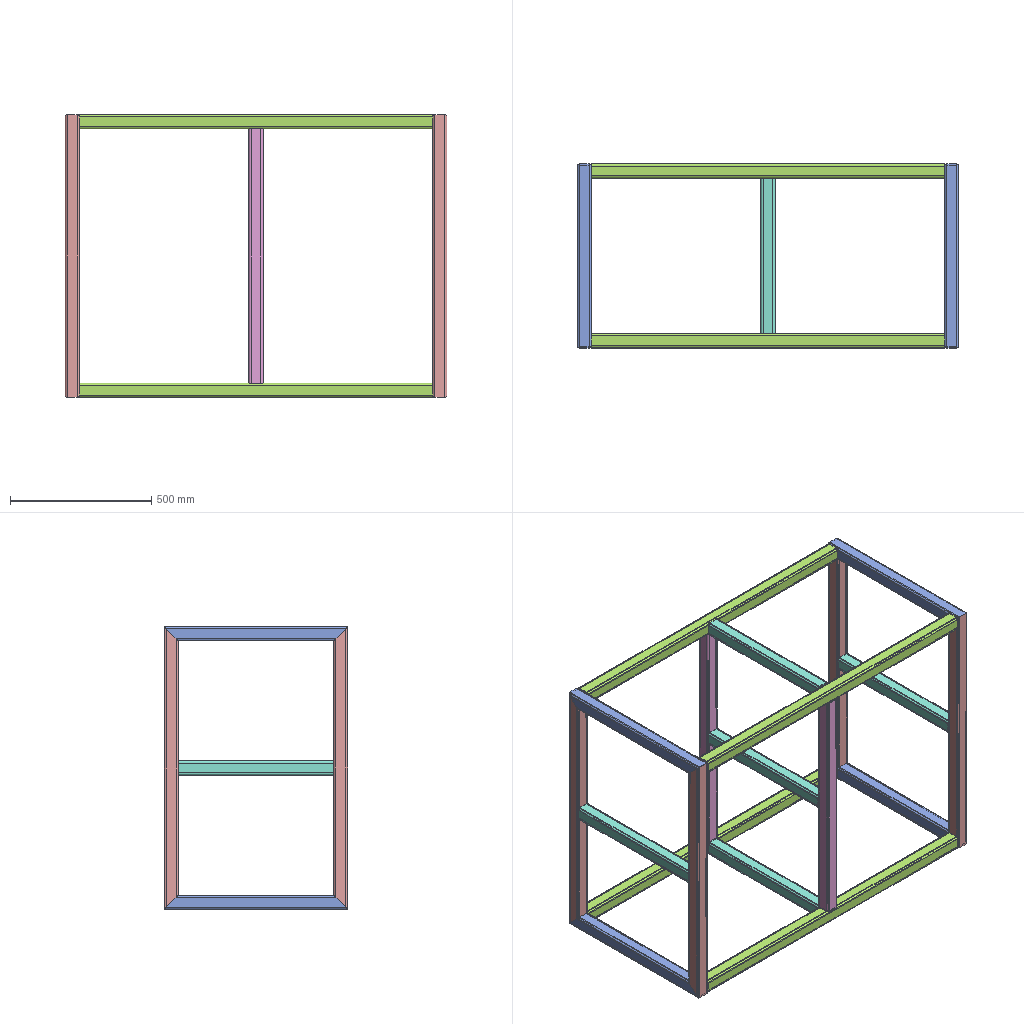Assembly | SolidWorks | 5 different items | 21 placed | box 1350 x 650 x 1000 mm
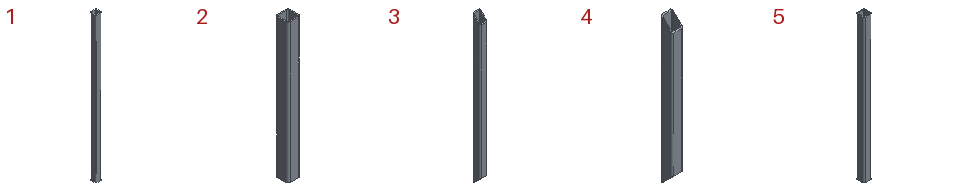Parts list (item | quantity | size | volume | features):
1 | x4 | 50 x 50 x 1250 mm | 868496 mm3 | features Extrusion 1
2 | x5 | 50 x 50 x 550 mm | 382138 mm3 | features Extrusion 1
3 | x6 | 50 x 50 x 1000 mm | 660057 mm3 | features Extrusion 1, ICE 1, MirrorPattern 1
4 | x4 | 50 x 50 x 650 mm | 416878 mm3 | features Extrusion 1, ICE 1, MirrorPattern 1
5 | x2 | 50 x 50 x 900 mm | 625317 mm3 | features Extrusion 1
Mates (type | each side: item.copy, entity, surface, feature):
Coincident | 3.1 face plane Boss-Extrude1 | 4.1 face plane Boss-Extrude1
Coincident | 3.1 face plane Mirror1 | 4.1 face plane Cut-Extrude1
Coincident | 3.1 edge | 4.1 edge
Coincident | 4.2 face plane Boss-Extrude1 | 1.1 face plane Boss-Extrude1 | 2 times
Coincident | 3.2 face plane Boss-Extrude1 | 1.1 face plane Boss-Extrude1
Coincident | 1.2 face plane Boss-Extrude1 | 5.1 face plane Boss-Extrude1 | 2 times
DistanceDim | 5.1 plane | 3.3 face plane Boss-Extrude1
Coincident | 3.4 face plane Boss-Extrude1 | 2.1 face plane Boss-Extrude1
Coincident | 3.2 face plane Boss-Extrude1 | 2.1 face plane Boss-Extrude1
DistanceDim | 2.1 plane | 4.2 face plane Boss-Extrude1
Coincident | 5.2 face plane Boss-Extrude1 | 2.2 face plane Boss-Extrude1 | 2 times
DistanceDim | 2.2 plane | 1.1 face plane Boss-Extrude1
Coincident | 1.1 face plane Boss-Extrude1 | 2.3 face plane Boss-Extrude1 | 2 times
Coincident | 5.1 face plane Boss-Extrude1 | 2.3 face plane Boss-Extrude1